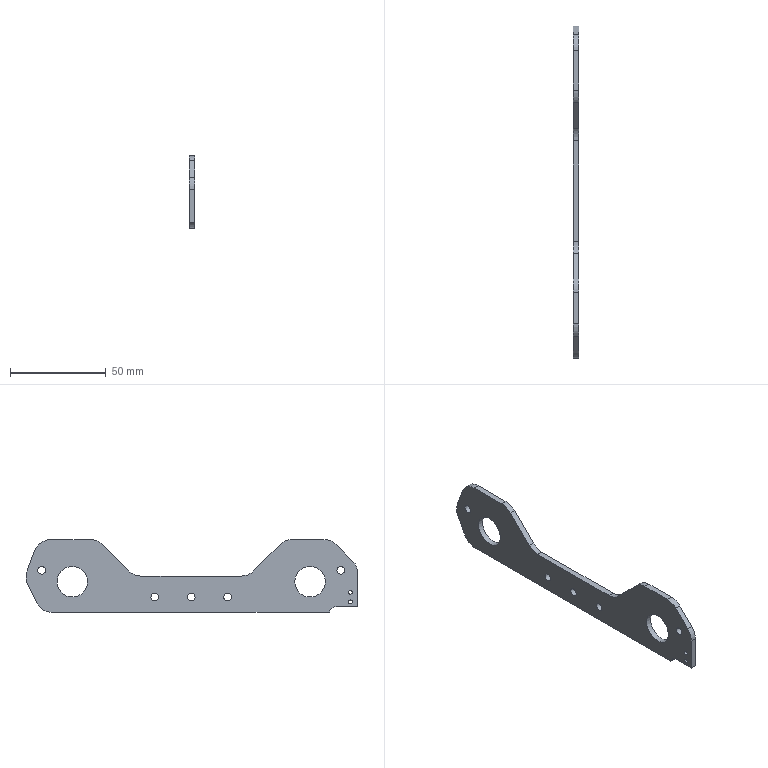Part | STEP file | 1-04.1 | 1 solid | 32 faces | box 3 x 173.195 x 38 mm | volume 12978 mm3 | cylinder 19 | plane 13 | commonest cylinder face diameters 18 x9 4 x5 2 x2 16 x2 8 x1